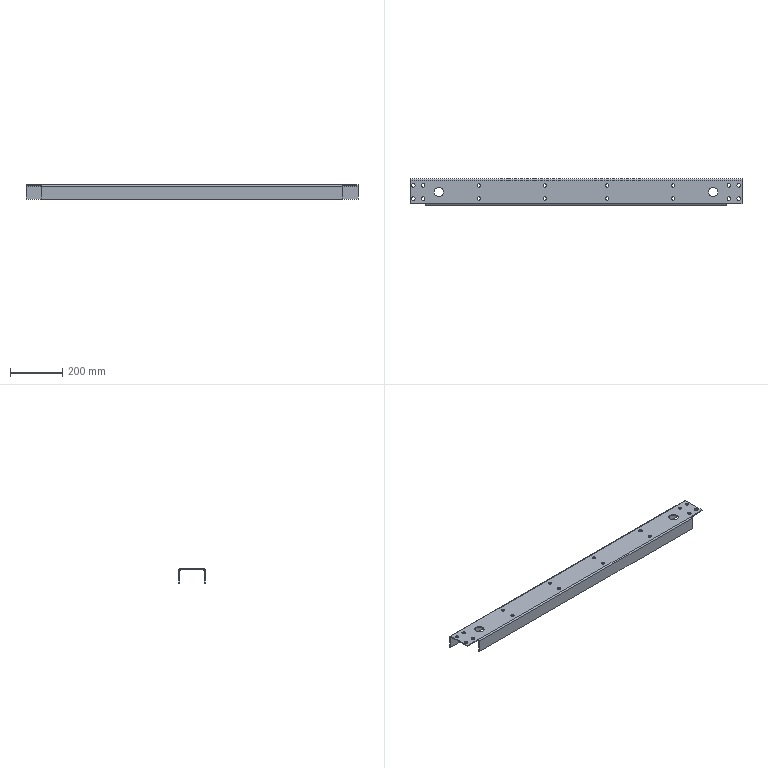Part | SolidWorks | features ICE 2, FlatPattern 1, SMBaseFlange 1, SheetMetal 1 | 1 solid | 62 faces | box 1268 x 100 x 54 mm | volume 958422 mm3 | cylinder 40 | plane 22 | commonest cylinder face diameters 13 x16 14 x16 35.5 x4 2 x2 10 x2